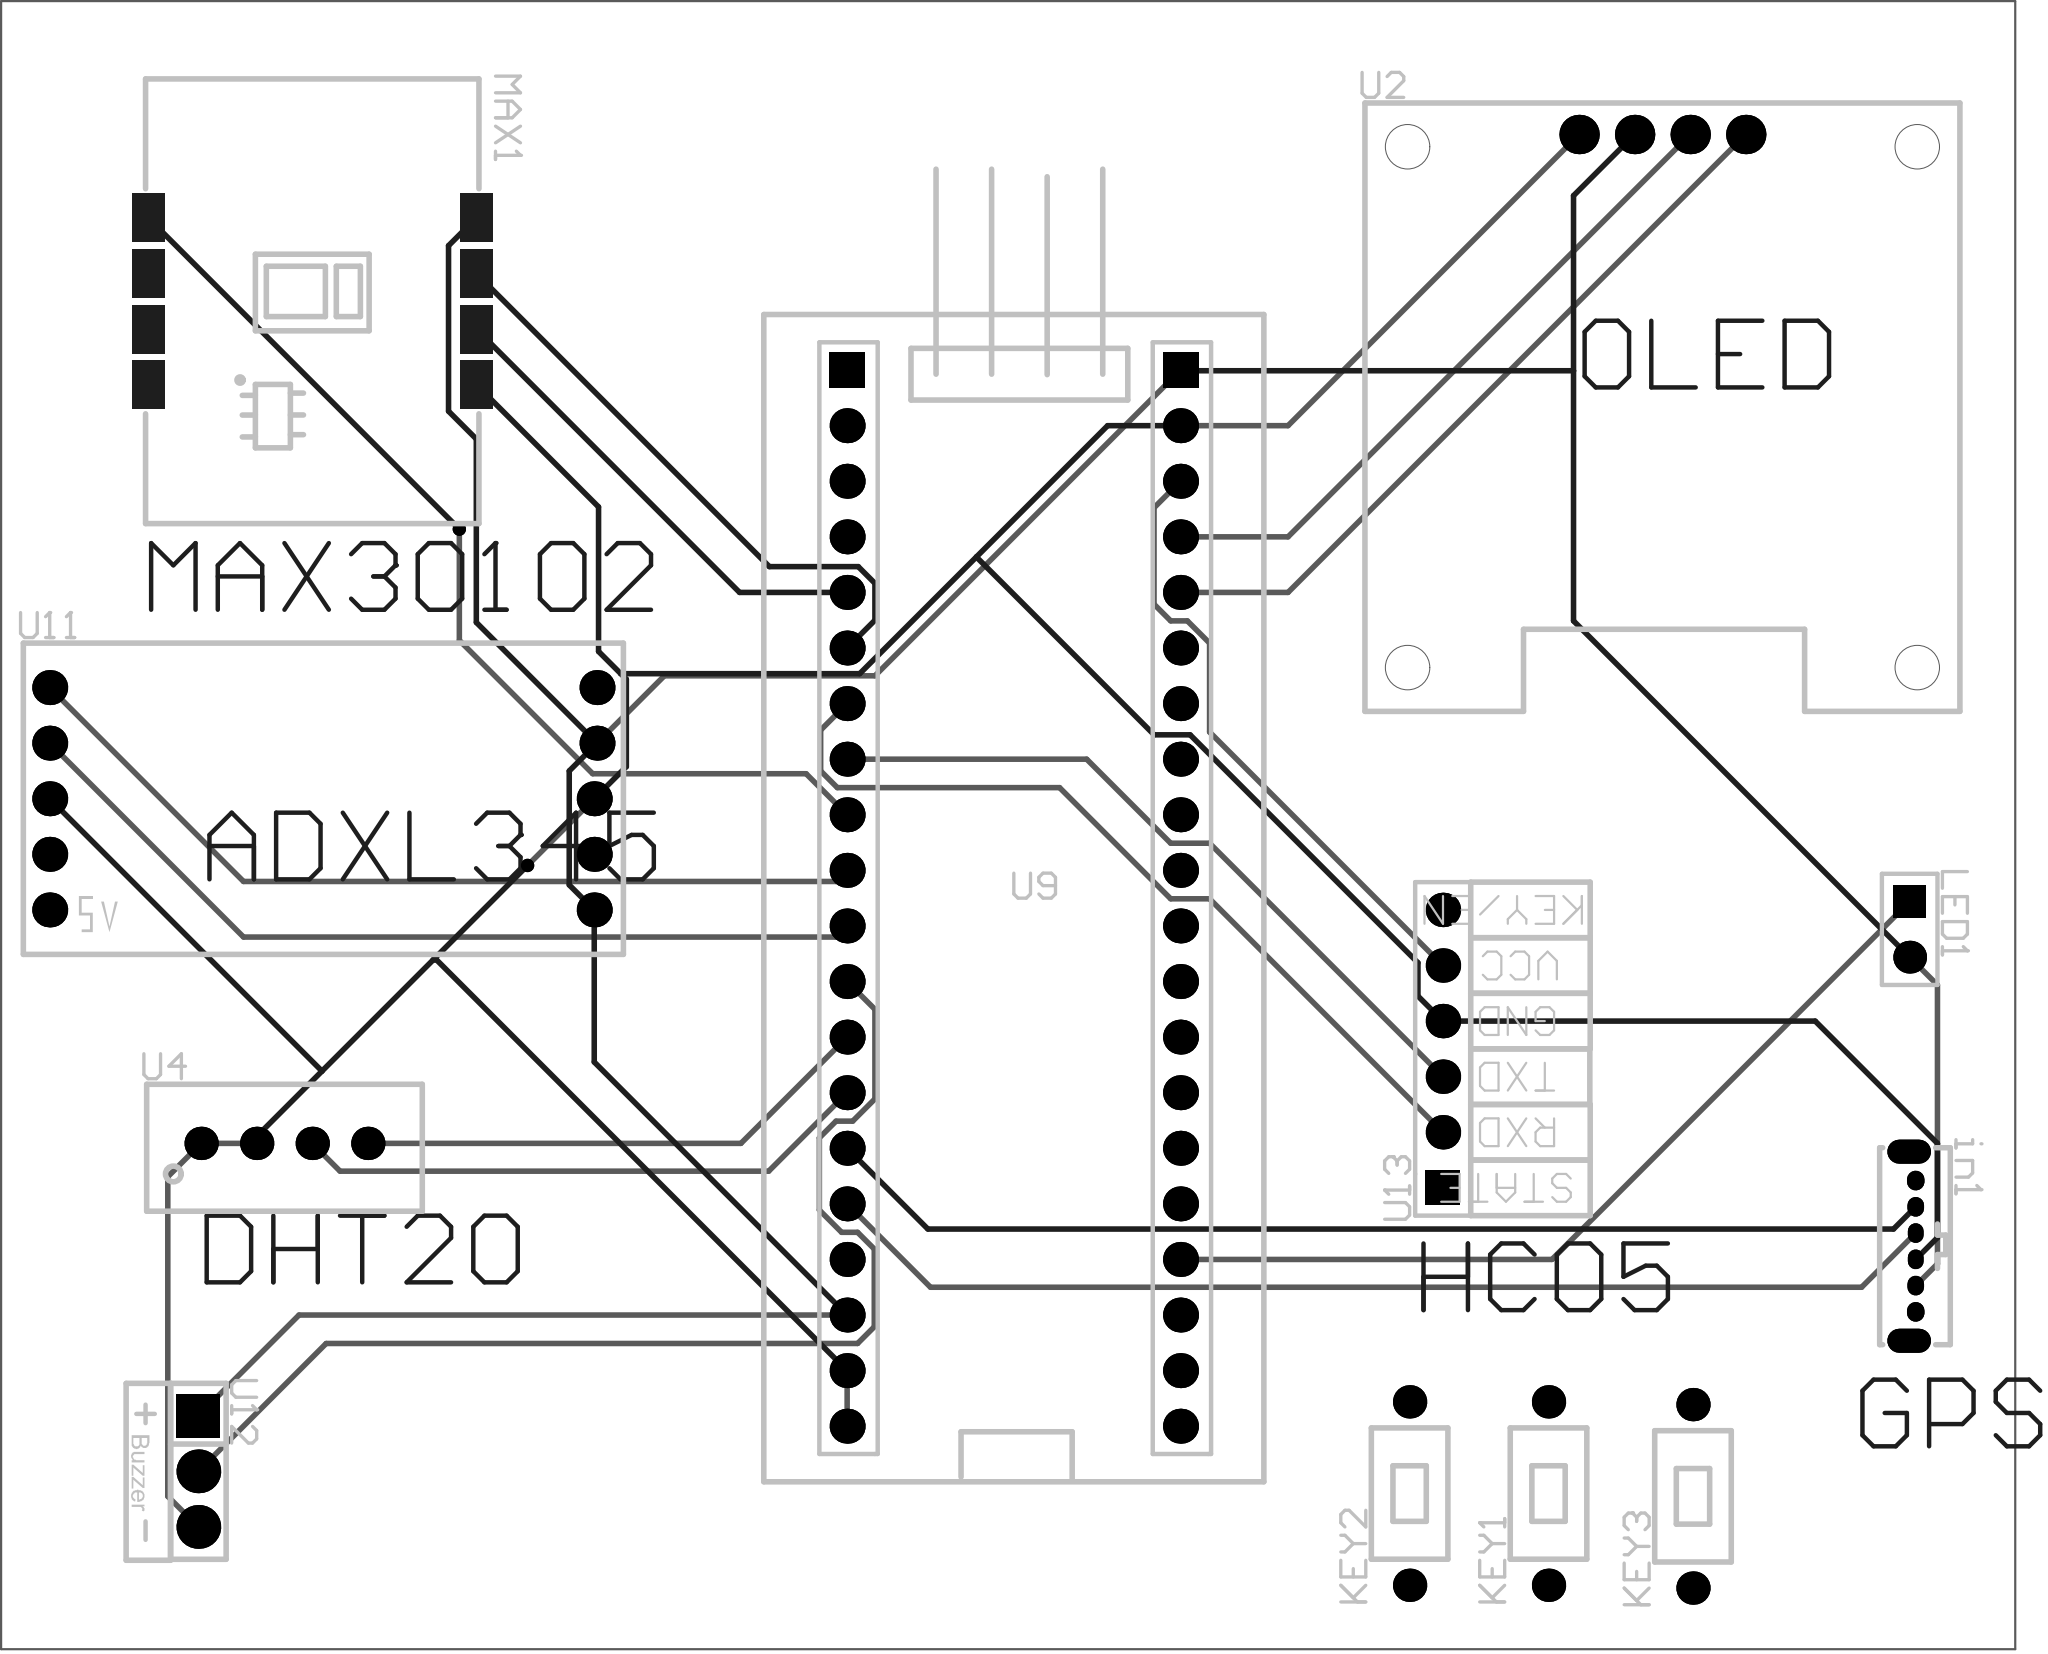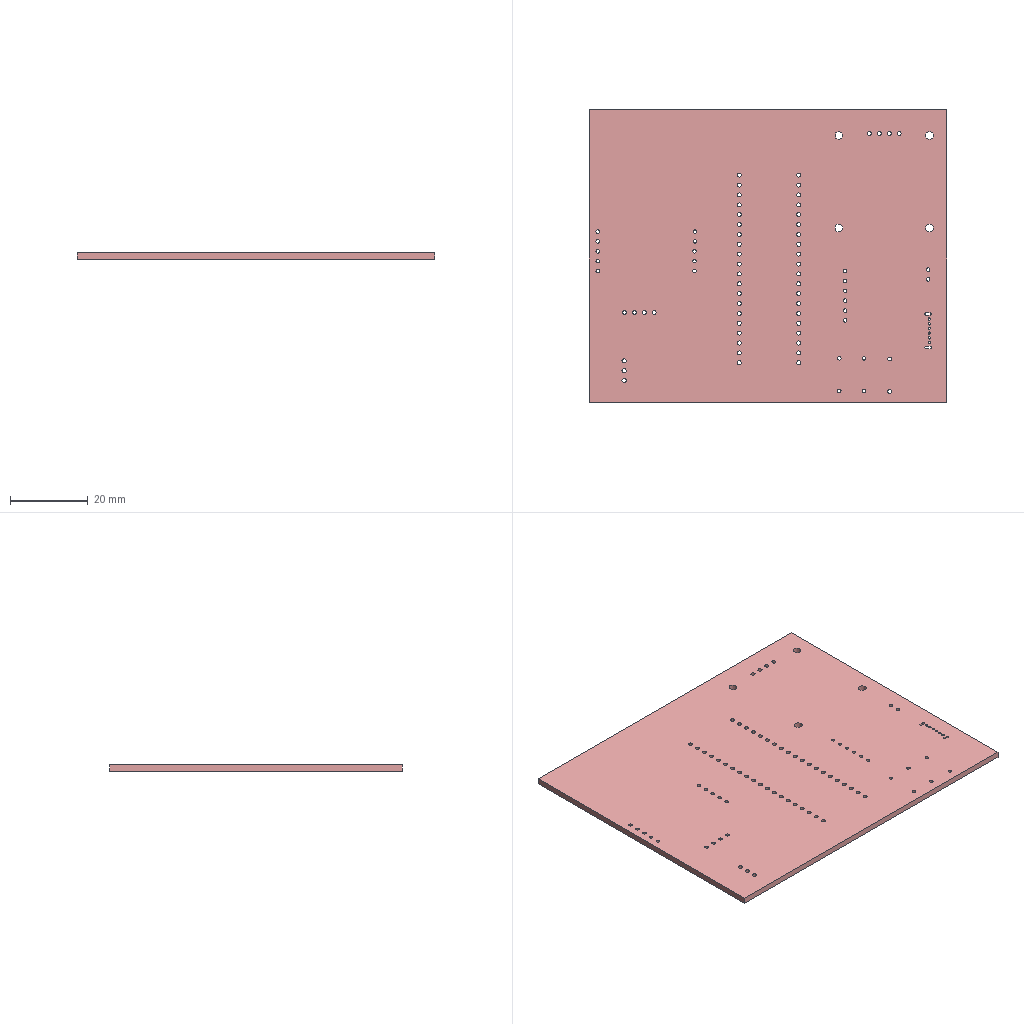Circuit board layout | Altium Designer | box 92.1 x 75.3 x 1.6 mm
Layer stack:
# Altium Designer layer stack of  (unit mm; dielectric type: 0 none, 1 core, 2 prepreg, 3 surface material)
index,name,kind,layer,copper_thickness_mm,dielectric_type,dielectric_thickness_mm,dielectric_material,dielectric_constant
0,Top Paste Mask Layer,other,,,,,,
1,Top Silkscreen Layer,other,,,,,,
2,Top Solder Mask Layer,dielectric,,,3,0.01,,3.3
3,Top Layer,copper,Top Layer,0.035,,,,
4,Dielectric1,dielectric,,,3,1.51,FR4,4.5
5,Bottom Layer,copper,Bottom Layer,0.035,,,,
6,Bottom Solder Mask Layer,dielectric,,,3,0.01,,3.3
7,Bottom Silkscreen Layer,other,,,,,,
8,Bottom Paste Mask Layer,other,,,,,,
# drill layer pairs: low layer,high layer
drill_pair,Top Layer,Bottom Layer
Part placement:
Designator,Comment,Layer,Footprint,Center-X(mm),Center-Y(mm),Rotation
KEY3,Through-hole tact switch,TopLayer,直插轻触开关3*6*5,153.543,83.185,90
KEY2,Through-hole tact switch,TopLayer,直插轻触开关3*6*5,140.589,83.312,90
KEY1,Through-hole tact switch,TopLayer,直插轻触开关3*6*5,146.939,83.312,90
MAX1,MAX30102 module,TopLayer,COMM-SMD_8P-L20.2-W15.4-P2.54_MAX30102,90.424,137.795,270
U2,0.96OLED,TopLayer,OLED-TH_L27.8-W27.2-P2.54_C9900033791,152.146,145.415,0
U4,DHT20,TopLayer,SENSOR-TH_DHT20,89.154,99.314,0
U9,STM32F103C8T6 minimum system board,TopLayer,STM32F103C8T6核心板,122.496,110.52,0
U11,ADXL345,TopLayer,COMM-TH_ADXL345,90.932,115.062,0
U12,Buzzer,TopLayer,蜂鸣器,85.217,84.328,270
U13,HC-05,TopLayer,HC05_6P,142.113,103.632,90
in1,gps,TopLayer,TYPE-C-6PIN-TH_C9900014686,163.576,94.615,270
LED1,LED,TopLayer,HDR1X2,163.449,109.093,270
Pad and via stacks:
# Altium Designer via and pad stacks of  (unit mm). Each distinct definition once, with the count of objects using it.
# via: kind,start_layer,end_layer,hole_mm,diameter_mm,mode(0 simple;1 top-mid-bottom;2 full stack),diameter_per_layer,count,example_net
# pad: kind,layer,hole_mm,hole_type(0 round;1 square;2 slot),plating,top_size,top_shape(1 round;2 rect;3 octagon;9 rounded rect),mid_size,bottom_size,mode,footprint,size_per_layer,count,example
pad,Multi-Layer,0.9144,0,plated,1.524x1.524,1,1.524x1.524,1.524x1.524,0,\u00D6\u00B1\u00B2\u00E5\u00C7\u00E1\u00B4\u00A5\u00BF\u00AA\u00B9\u00D83*6*5,,6,KEY3.2
pad,Multi-Layer,1.05,0,plated,1.8x1.8,1,1.8x1.8,1.8x1.8,0,OLED-TH_L27.8-W27.2-P2.54_C9900033791,,4,U2.1
pad,Multi-Layer,0.9144,0,plated,1.524x1.524,1,1.524x1.524,1.524x1.524,0,SENSOR-TH_DHT20,,4,U4.1
pad,Multi-Layer,1.049,0,plated,1.6x1.6,2,1.6x1.6,1.6x1.6,0,STM32F103C8T6\u00BA\u00CB\u00D0\u00C4\u00B0\u00E5,,2,U9.1
pad,Multi-Layer,1.049,0,plated,1.6x1.6,1,1.6x1.6,1.6x1.6,0,STM32F103C8T6\u00BA\u00CB\u00D0\u00C4\u00B0\u00E5,,38,U9.2
pad,Multi-Layer,0.9,0,plated,1.6x1.6,1,1.6x1.6,1.6x1.6,0,COMM-TH_ADXL345,,10,U11.1
pad,Multi-Layer,1.1,0,plated,2x2,2,2x2,2x2,0,\u00B7\u00E4\u00C3\u00F9\u00C6\u00F7,,1,U12.1
pad,Multi-Layer,1.1,0,plated,2x2,1,2x2,2x2,0,\u00B7\u00E4\u00C3\u00F9\u00C6\u00F7,,2,U12.2
pad,Multi-Layer,0.889,0,plated,1.575x1.575,1,1.575x1.575,1.575x1.575,0,HC05_6P,,5,U13.6
pad,Multi-Layer,0.889,0,plated,1.575x1.575,2,1.575x1.575,1.575x1.575,0,HC05_6P,,1,U13.1
pad,Multi-Layer,0.5,2,plated,0.9x0.76,1,0.9x0.76,0.9x0.76,0,TYPE-C-6PIN-TH_C9900014686,,2,in1.2
pad,Multi-Layer,0.6,2,plated,1.1x2,1,1.1x2,1.1x2,0,TYPE-C-6PIN-TH_C9900014686,,2,in1.7
pad,Multi-Layer,0.5,2,plated,0.9x0.8,1,0.9x0.8,0.9x0.8,0,TYPE-C-6PIN-TH_C9900014686,,2,in1.6
pad,Multi-Layer,0.5,2,plated,0.9x0.72,1,0.9x0.72,0.9x0.72,0,TYPE-C-6PIN-TH_C9900014686,,2,in1.4
pad,Multi-Layer,0.9,0,plated,1.5x1.5,1,1.5x1.5,1.5x1.5,0,HDR1X2,,1,LED1.2
pad,Multi-Layer,0.9,0,plated,1.5x1.5,2,1.5x1.5,1.5x1.5,0,HDR1X2,,1,LED1.1
pad,Top Layer,0,0,plated,2.2x1.5,2,2.2x1.5,2.2x1.5,0,COMM-SMD_8P-L20.2-W15.4-P2.54_MAX30102,,8,MAX1.8
via,Top Layer,Bottom Layer,0.3048,0.61,0,,2,PA4